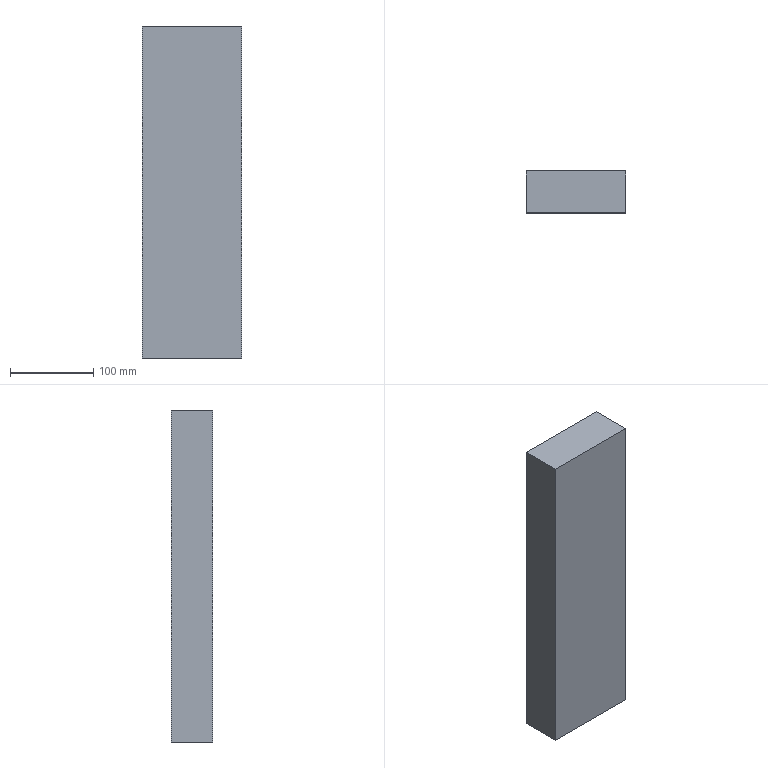Part | SolidWorks | features Extrusion 1 | 1 solid | 6 faces | box 120 x 50 x 400 mm | volume 2400000 mm3 | plane 6
STEP:
#1=CARTESIAN_POINT('',(0.,50.,0.));
#2=VERTEX_POINT('',#1);
#3=CARTESIAN_POINT('',(0.,0.,0.));
#4=VERTEX_POINT('',#3);
#5=CARTESIAN_POINT('',(0.,0.,0.));
#6=DIRECTION('',(0.,-1.,0.));
#7=VECTOR('',#6,1000.);
#8=LINE('',#5,#7);
#9=EDGE_CURVE('',#2,#4,#8,.T.);
#10=ORIENTED_EDGE('',*,*,#9,.T.);
#11=CARTESIAN_POINT('',(0.,0.,400.));
#12=VERTEX_POINT('',#11);
#13=CARTESIAN_POINT('',(0.,0.,400.));
#14=DIRECTION('',(0.,0.,-1.));
#15=VECTOR('',#14,1000.);
#16=LINE('',#13,#15);
#17=EDGE_CURVE('',#12,#4,#16,.T.);
#18=ORIENTED_EDGE('',*,*,#17,.F.);
#19=CARTESIAN_POINT('',(0.,50.,400.));
#20=VERTEX_POINT('',#19);
#21=CARTESIAN_POINT('',(0.,0.,400.));
#22=DIRECTION('',(0.,-1.,0.));
#23=VECTOR('',#22,1000.);
#24=LINE('',#21,#23);
#25=EDGE_CURVE('',#20,#12,#24,.T.);
#26=ORIENTED_EDGE('',*,*,#25,.F.);
#27=CARTESIAN_POINT('',(0.,50.,400.));
#28=DIRECTION('',(0.,0.,-1.));
#29=VECTOR('',#28,1000.);
#30=LINE('',#27,#29);
#31=EDGE_CURVE('',#20,#2,#30,.T.);
#32=ORIENTED_EDGE('',*,*,#31,.T.);
#33=EDGE_LOOP('',(#10,#18,#26,#32));
#34=FACE_OUTER_BOUND('',#33,.T.);
#35=CARTESIAN_POINT('',(0.,0.,400.));
#36=DIRECTION('',(1.,0.,0.));
#37=DIRECTION('',(0.,0.,-1.));
#38=AXIS2_PLACEMENT_3D('',#35,#36,#37);
#39=PLANE('',#38);
#40=ADVANCED_FACE('',(#34),#39,.F.);
#41=CARTESIAN_POINT('',(120.,0.,0.));
#42=VERTEX_POINT('',#41);
#43=CARTESIAN_POINT('',(0.,0.,0.));
#44=DIRECTION('',(1.,0.,0.));
#45=VECTOR('',#44,1000.);
#46=LINE('',#43,#45);
#47=EDGE_CURVE('',#4,#42,#46,.T.);
#48=ORIENTED_EDGE('',*,*,#47,.T.);
#49=CARTESIAN_POINT('',(120.,0.,400.));
#50=VERTEX_POINT('',#49);
#51=CARTESIAN_POINT('',(120.,0.,400.));
#52=DIRECTION('',(0.,0.,-1.));
#53=VECTOR('',#52,1000.);
#54=LINE('',#51,#53);
#55=EDGE_CURVE('',#50,#42,#54,.T.);
#56=ORIENTED_EDGE('',*,*,#55,.F.);
#57=CARTESIAN_POINT('',(0.,0.,400.));
#58=DIRECTION('',(1.,0.,0.));
#59=VECTOR('',#58,1000.);
#60=LINE('',#57,#59);
#61=EDGE_CURVE('',#12,#50,#60,.T.);
#62=ORIENTED_EDGE('',*,*,#61,.F.);
#63=ORIENTED_EDGE('',*,*,#17,.T.);
#64=EDGE_LOOP('',(#48,#56,#62,#63));
#65=FACE_OUTER_BOUND('',#64,.T.);
#66=CARTESIAN_POINT('',(0.,0.,400.));
#67=DIRECTION('',(0.,1.,0.));
#68=DIRECTION('',(0.,0.,1.));
#69=AXIS2_PLACEMENT_3D('',#66,#67,#68);
#70=PLANE('',#69);
#71=ADVANCED_FACE('',(#65),#70,.F.);
#72=CARTESIAN_POINT('',(120.,50.,0.));
#73=VERTEX_POINT('',#72);
#74=CARTESIAN_POINT('',(120.,0.,0.));
#75=DIRECTION('',(0.,1.,0.));
#76=VECTOR('',#75,1000.);
#77=LINE('',#74,#76);
#78=EDGE_CURVE('',#42,#73,#77,.T.);
#79=ORIENTED_EDGE('',*,*,#78,.T.);
#80=CARTESIAN_POINT('',(120.,50.,400.));
#81=VERTEX_POINT('',#80);
#82=CARTESIAN_POINT('',(120.,50.,400.));
#83=DIRECTION('',(0.,0.,-1.));
#84=VECTOR('',#83,1000.);
#85=LINE('',#82,#84);
#86=EDGE_CURVE('',#81,#73,#85,.T.);
#87=ORIENTED_EDGE('',*,*,#86,.F.);
#88=CARTESIAN_POINT('',(120.,0.,400.));
#89=DIRECTION('',(0.,1.,0.));
#90=VECTOR('',#89,1000.);
#91=LINE('',#88,#90);
#92=EDGE_CURVE('',#50,#81,#91,.T.);
#93=ORIENTED_EDGE('',*,*,#92,.F.);
#94=ORIENTED_EDGE('',*,*,#55,.T.);
#95=EDGE_LOOP('',(#79,#87,#93,#94));
#96=FACE_OUTER_BOUND('',#95,.T.);
#97=CARTESIAN_POINT('',(120.,0.,400.));
#98=DIRECTION('',(-1.,0.,0.));
#99=DIRECTION('',(0.,0.,1.));
#100=AXIS2_PLACEMENT_3D('',#97,#98,#99);
#101=PLANE('',#100);
#102=ADVANCED_FACE('',(#96),#101,.F.);
#103=CARTESIAN_POINT('',(0.,50.,0.));
#104=DIRECTION('',(-1.,0.,0.));
#105=VECTOR('',#104,1000.);
#106=LINE('',#103,#105);
#107=EDGE_CURVE('',#73,#2,#106,.T.);
#108=ORIENTED_EDGE('',*,*,#107,.T.);
#109=ORIENTED_EDGE('',*,*,#31,.F.);
#110=CARTESIAN_POINT('',(0.,50.,400.));
#111=DIRECTION('',(-1.,0.,0.));
#112=VECTOR('',#111,1000.);
#113=LINE('',#110,#112);
#114=EDGE_CURVE('',#81,#20,#113,.T.);
#115=ORIENTED_EDGE('',*,*,#114,.F.);
#116=ORIENTED_EDGE('',*,*,#86,.T.);
#117=EDGE_LOOP('',(#108,#109,#115,#116));
#118=FACE_OUTER_BOUND('',#117,.T.);
#119=CARTESIAN_POINT('',(0.,50.,400.));
#120=DIRECTION('',(0.,-1.,0.));
#121=DIRECTION('',(0.,0.,-1.));
#122=AXIS2_PLACEMENT_3D('',#119,#120,#121);
#123=PLANE('',#122);
#124=ADVANCED_FACE('',(#118),#123,.F.);
#125=ORIENTED_EDGE('',*,*,#25,.T.);
#126=ORIENTED_EDGE('',*,*,#61,.T.);
#127=ORIENTED_EDGE('',*,*,#92,.T.);
#128=ORIENTED_EDGE('',*,*,#114,.T.);
#129=EDGE_LOOP('',(#125,#126,#127,#128));
#130=FACE_OUTER_BOUND('',#129,.T.);
#131=CARTESIAN_POINT('',(0.,0.,400.));
#132=DIRECTION('',(0.,0.,-1.));
#133=DIRECTION('',(-1.,0.,0.));
#134=AXIS2_PLACEMENT_3D('',#131,#132,#133);
#135=PLANE('',#134);
#136=ADVANCED_FACE('',(#130),#135,.F.);
#137=ORIENTED_EDGE('',*,*,#9,.F.);
#138=ORIENTED_EDGE('',*,*,#107,.F.);
#139=ORIENTED_EDGE('',*,*,#78,.F.);
#140=ORIENTED_EDGE('',*,*,#47,.F.);
#141=EDGE_LOOP('',(#137,#138,#139,#140));
#142=FACE_OUTER_BOUND('',#141,.T.);
#143=CARTESIAN_POINT('',(0.,0.,0.));
#144=DIRECTION('',(0.,0.,-1.));
#145=DIRECTION('',(-1.,0.,0.));
#146=AXIS2_PLACEMENT_3D('',#143,#144,#145);
#147=PLANE('',#146);
#148=ADVANCED_FACE('',(#142),#147,.T.);
#149=CLOSED_SHELL('',(#40,#71,#102,#124,#136,#148));
#150=MANIFOLD_SOLID_BREP('',#149);
#151=CARTESIAN_POINT('',(0.,0.,0.));
#152=DIRECTION('',(0.,0.,1.));
#153=DIRECTION('',(1.,0.,0.));
#154=AXIS2_PLACEMENT_3D('',#151,#152,#153);
#155=(LENGTH_UNIT()NAMED_UNIT(*)SI_UNIT(.MILLI.,.METRE.));
#156=UNCERTAINTY_MEASURE_WITH_UNIT(LENGTH_MEASURE(0.00001),#155,'','');
#157=(NAMED_UNIT(*)PLANE_ANGLE_UNIT()SI_UNIT($,.RADIAN.));
#158=(NAMED_UNIT(*)SI_UNIT($,.STERADIAN.)SOLID_ANGLE_UNIT());
#159=(GEOMETRIC_REPRESENTATION_CONTEXT(3)GLOBAL_UNCERTAINTY_ASSIGNED_CONTEXT((#156))GLOBAL_UNIT_ASSIGNED_CONTEXT((#155,#157,#158))REPRESENTATION_CONTEXT('',''));
#160=ADVANCED_BREP_SHAPE_REPRESENTATION('',(#150,#154),#159);